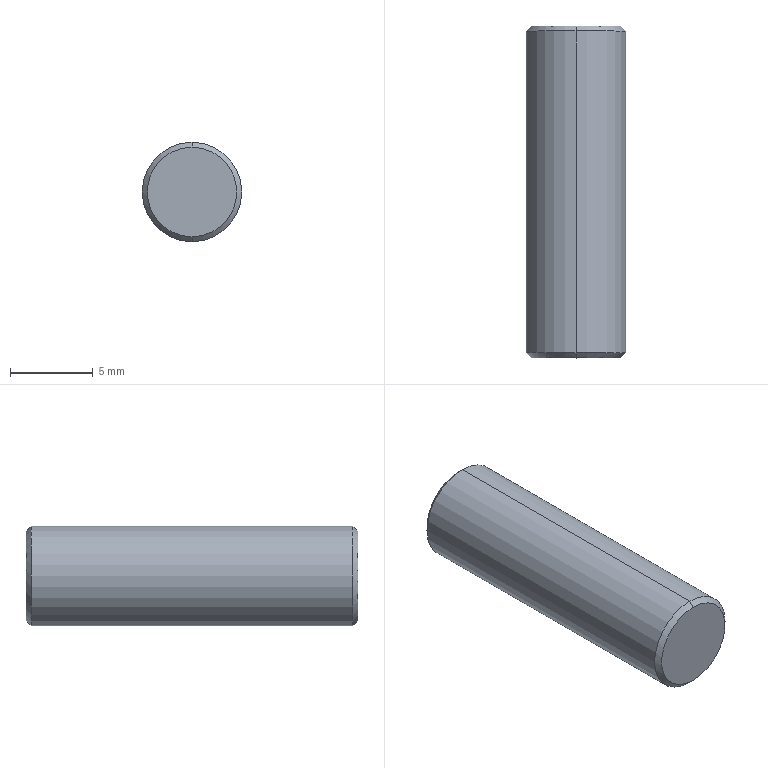Part | STEP file | PN_0030_default | 1 solid | 8 faces | box 6 x 20 x 6 mm | volume 563.847 mm3 | cone 4 | cylinder 2 | plane 2 | commonest cylinder face diameters 6 x2
STEP:
#1=CARTESIAN_POINT('',(0.,0.,0.));
#2=DIRECTION('',(0.,0.,1.));
#3=DIRECTION('',(1.,0.,0.));
#4=AXIS2_PLACEMENT_3D('',#1,#2,#3);
#5=CARTESIAN_POINT('',(0.,20.,2.7));
#6=VERTEX_POINT('',#5);
#7=CARTESIAN_POINT('',(0.,20.,-2.7));
#8=VERTEX_POINT('',#7);
#9=CARTESIAN_POINT('',(0.,20.,0.));
#10=DIRECTION('',(0.,1.,0.));
#11=DIRECTION('',(0.,0.,1.));
#12=AXIS2_PLACEMENT_3D('',#9,#10,#11);
#13=CIRCLE('',#12,2.7);
#14=CARTESIAN_POINT('',(0.,20.,0.));
#15=DIRECTION('',(0.,-1.,0.));
#16=DIRECTION('',(0.,0.,-1.));
#17=AXIS2_PLACEMENT_3D('',#14,#15,#16);
#18=CONICAL_SURFACE('',#17,2.7,0.7854);
#19=CARTESIAN_POINT('',(3.142,0.));
#20=DIRECTION('',(-1.,0.));
#21=VECTOR('',#20,1.);
#22=LINE('',#19,#21);
#23=(GEOMETRIC_REPRESENTATION_CONTEXT(2)PARAMETRIC_REPRESENTATION_CONTEXT()REPRESENTATION_CONTEXT('',''));
#24=DEFINITIONAL_REPRESENTATION('',(#22),#23);
#25=PCURVE('',#18,#24);
#26=CARTESIAN_POINT('',(0.,20.,0.));
#27=DIRECTION('',(0.,1.,0.));
#28=DIRECTION('',(0.,0.,1.));
#29=AXIS2_PLACEMENT_3D('',#26,#27,#28);
#30=PLANE('',#29);
#31=CARTESIAN_POINT('',(0.,0.));
#32=DIRECTION('',(1.,0.));
#33=AXIS2_PLACEMENT_2D('',#31,#32);
#34=CIRCLE('',#33,2.7);
#35=(GEOMETRIC_REPRESENTATION_CONTEXT(2)PARAMETRIC_REPRESENTATION_CONTEXT()REPRESENTATION_CONTEXT('',''));
#36=DEFINITIONAL_REPRESENTATION('',(#34),#35);
#37=PCURVE('',#30,#36);
#38=SURFACE_CURVE('',#13,(#25,#37),.PCURVE_S1.);
#39=EDGE_CURVE('',#6,#8,#38,.T.);
#40=ORIENTED_EDGE('',*,*,#39,.F.);
#41=CARTESIAN_POINT('',(0.,19.7,3.));
#42=VERTEX_POINT('',#41);
#43=CARTESIAN_POINT('',(0.,20.,2.7));
#44=DIRECTION('',(0.,-0.7071,0.7071));
#45=VECTOR('',#44,1.);
#46=LINE('',#43,#45);
#47=CARTESIAN_POINT('',(3.142,0.));
#48=DIRECTION('',(0.,1.));
#49=VECTOR('',#48,1.);
#50=LINE('',#47,#49);
#51=(GEOMETRIC_REPRESENTATION_CONTEXT(2)PARAMETRIC_REPRESENTATION_CONTEXT()REPRESENTATION_CONTEXT('',''));
#52=DEFINITIONAL_REPRESENTATION('',(#50),#51);
#53=PCURVE('',#18,#52);
#54=CARTESIAN_POINT('',(0.,20.,0.));
#55=DIRECTION('',(0.,-1.,0.));
#56=DIRECTION('',(0.,0.,-1.));
#57=AXIS2_PLACEMENT_3D('',#54,#55,#56);
#58=CONICAL_SURFACE('',#57,2.7,0.7854);
#59=CARTESIAN_POINT('',(3.142,0.));
#60=DIRECTION('',(0.,1.));
#61=VECTOR('',#60,1.);
#62=LINE('',#59,#61);
#63=(GEOMETRIC_REPRESENTATION_CONTEXT(2)PARAMETRIC_REPRESENTATION_CONTEXT()REPRESENTATION_CONTEXT('',''));
#64=DEFINITIONAL_REPRESENTATION('',(#62),#63);
#65=PCURVE('',#58,#64);
#66=SURFACE_CURVE('',#46,(#53,#65),.PCURVE_S1.);
#67=EDGE_CURVE('',#6,#42,#66,.T.);
#68=ORIENTED_EDGE('',*,*,#67,.T.);
#69=CARTESIAN_POINT('',(0.,19.7,-3.));
#70=VERTEX_POINT('',#69);
#71=CARTESIAN_POINT('',(0.,19.7,0.));
#72=DIRECTION('',(0.,-1.,0.));
#73=DIRECTION('',(0.,0.,1.));
#74=AXIS2_PLACEMENT_3D('',#71,#72,#73);
#75=CIRCLE('',#74,3.);
#76=CARTESIAN_POINT('',(-3.142,0.3));
#77=DIRECTION('',(1.,0.));
#78=VECTOR('',#77,1.);
#79=LINE('',#76,#78);
#80=(GEOMETRIC_REPRESENTATION_CONTEXT(2)PARAMETRIC_REPRESENTATION_CONTEXT()REPRESENTATION_CONTEXT('',''));
#81=DEFINITIONAL_REPRESENTATION('',(#79),#80);
#82=PCURVE('',#18,#81);
#83=CARTESIAN_POINT('',(0.,20.,0.));
#84=DIRECTION('',(0.,-1.,0.));
#85=DIRECTION('',(0.,0.,-1.));
#86=AXIS2_PLACEMENT_3D('',#83,#84,#85);
#87=CYLINDRICAL_SURFACE('',#86,3.);
#88=CARTESIAN_POINT('',(-3.142,0.3));
#89=DIRECTION('',(1.,0.));
#90=VECTOR('',#89,1.);
#91=LINE('',#88,#90);
#92=(GEOMETRIC_REPRESENTATION_CONTEXT(2)PARAMETRIC_REPRESENTATION_CONTEXT()REPRESENTATION_CONTEXT('',''));
#93=DEFINITIONAL_REPRESENTATION('',(#91),#92);
#94=PCURVE('',#87,#93);
#95=SURFACE_CURVE('',#75,(#82,#94),.PCURVE_S1.);
#96=EDGE_CURVE('',#70,#42,#95,.T.);
#97=ORIENTED_EDGE('',*,*,#96,.F.);
#98=CARTESIAN_POINT('',(0.,20.,-2.7));
#99=DIRECTION('',(0.,-0.7071,-0.7071));
#100=VECTOR('',#99,1.);
#101=LINE('',#98,#100);
#102=CARTESIAN_POINT('',(0.,0.));
#103=DIRECTION('',(0.,1.));
#104=VECTOR('',#103,1.);
#105=LINE('',#102,#104);
#106=(GEOMETRIC_REPRESENTATION_CONTEXT(2)PARAMETRIC_REPRESENTATION_CONTEXT()REPRESENTATION_CONTEXT('',''));
#107=DEFINITIONAL_REPRESENTATION('',(#105),#106);
#108=PCURVE('',#18,#107);
#109=CARTESIAN_POINT('',(6.283,0.));
#110=DIRECTION('',(0.,1.));
#111=VECTOR('',#110,1.);
#112=LINE('',#109,#111);
#113=(GEOMETRIC_REPRESENTATION_CONTEXT(2)PARAMETRIC_REPRESENTATION_CONTEXT()REPRESENTATION_CONTEXT('',''));
#114=DEFINITIONAL_REPRESENTATION('',(#112),#113);
#115=PCURVE('',#58,#114);
#116=SURFACE_CURVE('',#101,(#108,#115),.PCURVE_S1.);
#117=EDGE_CURVE('',#8,#70,#116,.T.);
#118=ORIENTED_EDGE('',*,*,#117,.F.);
#119=EDGE_LOOP('',(#40,#68,#97,#118));
#120=FACE_BOUND('',#119,.T.);
#121=ADVANCED_FACE('',(#120),#18,.T.);
#122=CARTESIAN_POINT('',(0.,0.,-2.7));
#123=VERTEX_POINT('',#122);
#124=CARTESIAN_POINT('',(0.,0.,2.7));
#125=VERTEX_POINT('',#124);
#126=CARTESIAN_POINT('',(0.,0.,0.));
#127=DIRECTION('',(0.,-1.,0.));
#128=DIRECTION('',(0.,0.,1.));
#129=AXIS2_PLACEMENT_3D('',#126,#127,#128);
#130=CIRCLE('',#129,2.7);
#131=CARTESIAN_POINT('',(0.,0.3,0.));
#132=DIRECTION('',(0.,1.,0.));
#133=DIRECTION('',(0.,0.,1.));
#134=AXIS2_PLACEMENT_3D('',#131,#132,#133);
#135=CONICAL_SURFACE('',#134,3.,0.7854);
#136=CARTESIAN_POINT('',(6.283,-0.3));
#137=DIRECTION('',(-1.,0.));
#138=VECTOR('',#137,1.);
#139=LINE('',#136,#138);
#140=(GEOMETRIC_REPRESENTATION_CONTEXT(2)PARAMETRIC_REPRESENTATION_CONTEXT()REPRESENTATION_CONTEXT('',''));
#141=DEFINITIONAL_REPRESENTATION('',(#139),#140);
#142=PCURVE('',#135,#141);
#143=CARTESIAN_POINT('',(0.,0.,0.));
#144=DIRECTION('',(0.,1.,0.));
#145=DIRECTION('',(0.,0.,1.));
#146=AXIS2_PLACEMENT_3D('',#143,#144,#145);
#147=PLANE('',#146);
#148=CARTESIAN_POINT('',(2.7,0.));
#149=CARTESIAN_POINT('',(2.7,-4.677));
#150=CARTESIAN_POINT('',(-1.35,-2.338));
#151=CARTESIAN_POINT('',(-5.4,0.));
#152=CARTESIAN_POINT('',(-1.35,2.338));
#153=CARTESIAN_POINT('',(2.7,4.677));
#154=CARTESIAN_POINT('',(2.7,0.));
#155=(BOUNDED_CURVE()B_SPLINE_CURVE(2,(#148,#149,#150,#151,#152,#153,#154),.UNSPECIFIED.,.T.,.F.)B_SPLINE_CURVE_WITH_KNOTS((1,2,2,2,2,1),(-2.094,0.,2.094,4.189,6.283,8.378),.UNSPECIFIED.)CURVE()GEOMETRIC_REPRESENTATION_ITEM()RATIONAL_B_SPLINE_CURVE((1.,0.5,1.,0.5,1.,0.5,1.))REPRESENTATION_ITEM(''));
#156=(GEOMETRIC_REPRESENTATION_CONTEXT(2)PARAMETRIC_REPRESENTATION_CONTEXT()REPRESENTATION_CONTEXT('',''));
#157=DEFINITIONAL_REPRESENTATION('',(#155),#156);
#158=PCURVE('',#147,#157);
#159=SURFACE_CURVE('',#130,(#142,#158),.PCURVE_S1.);
#160=EDGE_CURVE('',#123,#125,#159,.T.);
#161=ORIENTED_EDGE('',*,*,#160,.F.);
#162=CARTESIAN_POINT('',(0.,0.3,-3.));
#163=VERTEX_POINT('',#162);
#164=CARTESIAN_POINT('',(0.,0.3,-3.));
#165=DIRECTION('',(0.,0.7071,-0.7071));
#166=VECTOR('',#165,1.);
#167=LINE('',#164,#166);
#168=CARTESIAN_POINT('',(3.142,0.));
#169=DIRECTION('',(0.,1.));
#170=VECTOR('',#169,1.);
#171=LINE('',#168,#170);
#172=(GEOMETRIC_REPRESENTATION_CONTEXT(2)PARAMETRIC_REPRESENTATION_CONTEXT()REPRESENTATION_CONTEXT('',''));
#173=DEFINITIONAL_REPRESENTATION('',(#171),#172);
#174=PCURVE('',#135,#173);
#175=CARTESIAN_POINT('',(0.,0.3,0.));
#176=DIRECTION('',(0.,1.,0.));
#177=DIRECTION('',(0.,0.,1.));
#178=AXIS2_PLACEMENT_3D('',#175,#176,#177);
#179=CONICAL_SURFACE('',#178,3.,0.7854);
#180=CARTESIAN_POINT('',(3.142,0.));
#181=DIRECTION('',(0.,1.));
#182=VECTOR('',#181,1.);
#183=LINE('',#180,#182);
#184=(GEOMETRIC_REPRESENTATION_CONTEXT(2)PARAMETRIC_REPRESENTATION_CONTEXT()REPRESENTATION_CONTEXT('',''));
#185=DEFINITIONAL_REPRESENTATION('',(#183),#184);
#186=PCURVE('',#179,#185);
#187=SURFACE_CURVE('',#167,(#174,#186),.PCURVE_S1.);
#188=EDGE_CURVE('',#123,#163,#187,.T.);
#189=ORIENTED_EDGE('',*,*,#188,.T.);
#190=CARTESIAN_POINT('',(0.,0.3,3.));
#191=VERTEX_POINT('',#190);
#192=CARTESIAN_POINT('',(0.,0.3,0.));
#193=DIRECTION('',(0.,1.,0.));
#194=DIRECTION('',(0.,0.,1.));
#195=AXIS2_PLACEMENT_3D('',#192,#193,#194);
#196=CIRCLE('',#195,3.);
#197=CARTESIAN_POINT('',(0.,0.));
#198=DIRECTION('',(1.,0.));
#199=VECTOR('',#198,1.);
#200=LINE('',#197,#199);
#201=(GEOMETRIC_REPRESENTATION_CONTEXT(2)PARAMETRIC_REPRESENTATION_CONTEXT()REPRESENTATION_CONTEXT('',''));
#202=DEFINITIONAL_REPRESENTATION('',(#200),#201);
#203=PCURVE('',#135,#202);
#204=CARTESIAN_POINT('',(3.142,19.7));
#205=DIRECTION('',(-1.,0.));
#206=VECTOR('',#205,1.);
#207=LINE('',#204,#206);
#208=(GEOMETRIC_REPRESENTATION_CONTEXT(2)PARAMETRIC_REPRESENTATION_CONTEXT()REPRESENTATION_CONTEXT('',''));
#209=DEFINITIONAL_REPRESENTATION('',(#207),#208);
#210=PCURVE('',#87,#209);
#211=SURFACE_CURVE('',#196,(#203,#210),.PCURVE_S1.);
#212=EDGE_CURVE('',#191,#163,#211,.T.);
#213=ORIENTED_EDGE('',*,*,#212,.F.);
#214=CARTESIAN_POINT('',(0.,0.3,3.));
#215=DIRECTION('',(0.,0.7071,0.7071));
#216=VECTOR('',#215,1.);
#217=LINE('',#214,#216);
#218=CARTESIAN_POINT('',(0.,0.));
#219=DIRECTION('',(0.,1.));
#220=VECTOR('',#219,1.);
#221=LINE('',#218,#220);
#222=(GEOMETRIC_REPRESENTATION_CONTEXT(2)PARAMETRIC_REPRESENTATION_CONTEXT()REPRESENTATION_CONTEXT('',''));
#223=DEFINITIONAL_REPRESENTATION('',(#221),#222);
#224=PCURVE('',#135,#223);
#225=CARTESIAN_POINT('',(6.283,0.));
#226=DIRECTION('',(0.,1.));
#227=VECTOR('',#226,1.);
#228=LINE('',#225,#227);
#229=(GEOMETRIC_REPRESENTATION_CONTEXT(2)PARAMETRIC_REPRESENTATION_CONTEXT()REPRESENTATION_CONTEXT('',''));
#230=DEFINITIONAL_REPRESENTATION('',(#228),#229);
#231=PCURVE('',#179,#230);
#232=SURFACE_CURVE('',#217,(#224,#231),.PCURVE_S1.);
#233=EDGE_CURVE('',#125,#191,#232,.T.);
#234=ORIENTED_EDGE('',*,*,#233,.F.);
#235=EDGE_LOOP('',(#161,#189,#213,#234));
#236=FACE_BOUND('',#235,.T.);
#237=ADVANCED_FACE('',(#236),#135,.T.);
#238=ORIENTED_EDGE('',*,*,#96,.T.);
#239=CARTESIAN_POINT('',(0.,20.,3.));
#240=DIRECTION('',(0.,-1.,0.));
#241=VECTOR('',#240,1.);
#242=LINE('',#239,#241);
#243=CARTESIAN_POINT('',(3.142,0.));
#244=DIRECTION('',(0.,1.));
#245=VECTOR('',#244,1.);
#246=LINE('',#243,#245);
#247=(GEOMETRIC_REPRESENTATION_CONTEXT(2)PARAMETRIC_REPRESENTATION_CONTEXT()REPRESENTATION_CONTEXT('',''));
#248=DEFINITIONAL_REPRESENTATION('',(#246),#247);
#249=PCURVE('',#87,#248);
#250=CARTESIAN_POINT('',(0.,20.,0.));
#251=DIRECTION('',(0.,-1.,0.));
#252=DIRECTION('',(0.,0.,-1.));
#253=AXIS2_PLACEMENT_3D('',#250,#251,#252);
#254=CYLINDRICAL_SURFACE('',#253,3.);
#255=CARTESIAN_POINT('',(3.142,0.));
#256=DIRECTION('',(0.,1.));
#257=VECTOR('',#256,1.);
#258=LINE('',#255,#257);
#259=(GEOMETRIC_REPRESENTATION_CONTEXT(2)PARAMETRIC_REPRESENTATION_CONTEXT()REPRESENTATION_CONTEXT('',''));
#260=DEFINITIONAL_REPRESENTATION('',(#258),#259);
#261=PCURVE('',#254,#260);
#262=SURFACE_CURVE('',#242,(#249,#261),.PCURVE_S1.);
#263=EDGE_CURVE('',#42,#191,#262,.T.);
#264=ORIENTED_EDGE('',*,*,#263,.T.);
#265=ORIENTED_EDGE('',*,*,#212,.T.);
#266=CARTESIAN_POINT('',(0.,20.,-3.));
#267=DIRECTION('',(0.,-1.,0.));
#268=VECTOR('',#267,1.);
#269=LINE('',#266,#268);
#270=CARTESIAN_POINT('',(0.,0.));
#271=DIRECTION('',(0.,1.));
#272=VECTOR('',#271,1.);
#273=LINE('',#270,#272);
#274=(GEOMETRIC_REPRESENTATION_CONTEXT(2)PARAMETRIC_REPRESENTATION_CONTEXT()REPRESENTATION_CONTEXT('',''));
#275=DEFINITIONAL_REPRESENTATION('',(#273),#274);
#276=PCURVE('',#87,#275);
#277=CARTESIAN_POINT('',(6.283,0.));
#278=DIRECTION('',(0.,1.));
#279=VECTOR('',#278,1.);
#280=LINE('',#277,#279);
#281=(GEOMETRIC_REPRESENTATION_CONTEXT(2)PARAMETRIC_REPRESENTATION_CONTEXT()REPRESENTATION_CONTEXT('',''));
#282=DEFINITIONAL_REPRESENTATION('',(#280),#281);
#283=PCURVE('',#254,#282);
#284=SURFACE_CURVE('',#269,(#276,#283),.PCURVE_S1.);
#285=EDGE_CURVE('',#70,#163,#284,.T.);
#286=ORIENTED_EDGE('',*,*,#285,.F.);
#287=EDGE_LOOP('',(#238,#264,#265,#286));
#288=FACE_BOUND('',#287,.T.);
#289=ADVANCED_FACE('',(#288),#87,.T.);
#290=ORIENTED_EDGE('',*,*,#263,.F.);
#291=CARTESIAN_POINT('',(0.,19.7,0.));
#292=DIRECTION('',(0.,-1.,0.));
#293=DIRECTION('',(0.,0.,1.));
#294=AXIS2_PLACEMENT_3D('',#291,#292,#293);
#295=CIRCLE('',#294,3.);
#296=CARTESIAN_POINT('',(3.142,0.3));
#297=DIRECTION('',(1.,0.));
#298=VECTOR('',#297,1.);
#299=LINE('',#296,#298);
#300=(GEOMETRIC_REPRESENTATION_CONTEXT(2)PARAMETRIC_REPRESENTATION_CONTEXT()REPRESENTATION_CONTEXT('',''));
#301=DEFINITIONAL_REPRESENTATION('',(#299),#300);
#302=PCURVE('',#254,#301);
#303=CARTESIAN_POINT('',(3.142,0.3));
#304=DIRECTION('',(1.,0.));
#305=VECTOR('',#304,1.);
#306=LINE('',#303,#305);
#307=(GEOMETRIC_REPRESENTATION_CONTEXT(2)PARAMETRIC_REPRESENTATION_CONTEXT()REPRESENTATION_CONTEXT('',''));
#308=DEFINITIONAL_REPRESENTATION('',(#306),#307);
#309=PCURVE('',#58,#308);
#310=SURFACE_CURVE('',#295,(#302,#309),.PCURVE_S1.);
#311=EDGE_CURVE('',#42,#70,#310,.T.);
#312=ORIENTED_EDGE('',*,*,#311,.T.);
#313=ORIENTED_EDGE('',*,*,#285,.T.);
#314=CARTESIAN_POINT('',(0.,0.3,0.));
#315=DIRECTION('',(0.,1.,0.));
#316=DIRECTION('',(0.,0.,1.));
#317=AXIS2_PLACEMENT_3D('',#314,#315,#316);
#318=CIRCLE('',#317,3.);
#319=CARTESIAN_POINT('',(9.425,19.7));
#320=DIRECTION('',(-1.,0.));
#321=VECTOR('',#320,1.);
#322=LINE('',#319,#321);
#323=(GEOMETRIC_REPRESENTATION_CONTEXT(2)PARAMETRIC_REPRESENTATION_CONTEXT()REPRESENTATION_CONTEXT('',''));
#324=DEFINITIONAL_REPRESENTATION('',(#322),#323);
#325=PCURVE('',#254,#324);
#326=CARTESIAN_POINT('',(0.,0.));
#327=DIRECTION('',(1.,0.));
#328=VECTOR('',#327,1.);
#329=LINE('',#326,#328);
#330=(GEOMETRIC_REPRESENTATION_CONTEXT(2)PARAMETRIC_REPRESENTATION_CONTEXT()REPRESENTATION_CONTEXT('',''));
#331=DEFINITIONAL_REPRESENTATION('',(#329),#330);
#332=PCURVE('',#179,#331);
#333=SURFACE_CURVE('',#318,(#325,#332),.PCURVE_S1.);
#334=EDGE_CURVE('',#163,#191,#333,.T.);
#335=ORIENTED_EDGE('',*,*,#334,.T.);
#336=EDGE_LOOP('',(#290,#312,#313,#335));
#337=FACE_BOUND('',#336,.T.);
#338=ADVANCED_FACE('',(#337),#254,.T.);
#339=CARTESIAN_POINT('',(0.,20.,0.));
#340=DIRECTION('',(0.,1.,0.));
#341=DIRECTION('',(0.,0.,1.));
#342=AXIS2_PLACEMENT_3D('',#339,#340,#341);
#343=CIRCLE('',#342,2.7);
#344=CARTESIAN_POINT('',(0.,0.));
#345=DIRECTION('',(1.,0.));
#346=AXIS2_PLACEMENT_2D('',#344,#345);
#347=CIRCLE('',#346,2.7);
#348=(GEOMETRIC_REPRESENTATION_CONTEXT(2)PARAMETRIC_REPRESENTATION_CONTEXT()REPRESENTATION_CONTEXT('',''));
#349=DEFINITIONAL_REPRESENTATION('',(#347),#348);
#350=PCURVE('',#30,#349);
#351=CARTESIAN_POINT('',(9.425,0.));
#352=DIRECTION('',(-1.,0.));
#353=VECTOR('',#352,1.);
#354=LINE('',#351,#353);
#355=(GEOMETRIC_REPRESENTATION_CONTEXT(2)PARAMETRIC_REPRESENTATION_CONTEXT()REPRESENTATION_CONTEXT('',''));
#356=DEFINITIONAL_REPRESENTATION('',(#354),#355);
#357=PCURVE('',#58,#356);
#358=SURFACE_CURVE('',#343,(#350,#357),.PCURVE_S1.);
#359=EDGE_CURVE('',#8,#6,#358,.T.);
#360=ORIENTED_EDGE('',*,*,#359,.T.);
#361=ORIENTED_EDGE('',*,*,#39,.T.);
#362=EDGE_LOOP('',(#360,#361));
#363=FACE_BOUND('',#362,.T.);
#364=ADVANCED_FACE('',(#363),#30,.T.);
#365=CARTESIAN_POINT('',(0.,0.,0.));
#366=DIRECTION('',(0.,-1.,0.));
#367=DIRECTION('',(0.,0.,1.));
#368=AXIS2_PLACEMENT_3D('',#365,#366,#367);
#369=CIRCLE('',#368,2.7);
#370=CARTESIAN_POINT('',(2.7,0.));
#371=CARTESIAN_POINT('',(2.7,-4.677));
#372=CARTESIAN_POINT('',(-1.35,-2.338));
#373=CARTESIAN_POINT('',(-5.4,0.));
#374=CARTESIAN_POINT('',(-1.35,2.338));
#375=CARTESIAN_POINT('',(2.7,4.677));
#376=CARTESIAN_POINT('',(2.7,0.));
#377=(BOUNDED_CURVE()B_SPLINE_CURVE(2,(#370,#371,#372,#373,#374,#375,#376),.UNSPECIFIED.,.T.,.F.)B_SPLINE_CURVE_WITH_KNOTS((1,2,2,2,2,1),(-2.094,0.,2.094,4.189,6.283,8.378),.UNSPECIFIED.)CURVE()GEOMETRIC_REPRESENTATION_ITEM()RATIONAL_B_SPLINE_CURVE((1.,0.5,1.,0.5,1.,0.5,1.))REPRESENTATION_ITEM(''));
#378=(GEOMETRIC_REPRESENTATION_CONTEXT(2)PARAMETRIC_REPRESENTATION_CONTEXT()REPRESENTATION_CONTEXT('',''));
#379=DEFINITIONAL_REPRESENTATION('',(#377),#378);
#380=PCURVE('',#147,#379);
#381=CARTESIAN_POINT('',(6.283,-0.3));
#382=DIRECTION('',(-1.,0.));
#383=VECTOR('',#382,1.);
#384=LINE('',#381,#383);
#385=(GEOMETRIC_REPRESENTATION_CONTEXT(2)PARAMETRIC_REPRESENTATION_CONTEXT()REPRESENTATION_CONTEXT('',''));
#386=DEFINITIONAL_REPRESENTATION('',(#384),#385);
#387=PCURVE('',#179,#386);
#388=SURFACE_CURVE('',#369,(#380,#387),.PCURVE_S1.);
#389=EDGE_CURVE('',#125,#123,#388,.T.);
#390=ORIENTED_EDGE('',*,*,#389,.T.);
#391=ORIENTED_EDGE('',*,*,#160,.T.);
#392=EDGE_LOOP('',(#390,#391));
#393=FACE_BOUND('',#392,.T.);
#394=ADVANCED_FACE('',(#393),#147,.F.);
#395=ORIENTED_EDGE('',*,*,#188,.F.);
#396=ORIENTED_EDGE('',*,*,#389,.F.);
#397=ORIENTED_EDGE('',*,*,#233,.T.);
#398=ORIENTED_EDGE('',*,*,#334,.F.);
#399=EDGE_LOOP('',(#395,#396,#397,#398));
#400=FACE_BOUND('',#399,.T.);
#401=ADVANCED_FACE('',(#400),#179,.T.);
#402=ORIENTED_EDGE('',*,*,#67,.F.);
#403=ORIENTED_EDGE('',*,*,#359,.F.);
#404=ORIENTED_EDGE('',*,*,#117,.T.);
#405=ORIENTED_EDGE('',*,*,#311,.F.);
#406=EDGE_LOOP('',(#402,#403,#404,#405));
#407=FACE_BOUND('',#406,.T.);
#408=ADVANCED_FACE('',(#407),#58,.T.);
#409=CLOSED_SHELL('',(#121,#237,#289,#338,#364,#394,#401,#408));
#410=MANIFOLD_SOLID_BREP('',#409);
#411=(LENGTH_UNIT()NAMED_UNIT(*)SI_UNIT(.MILLI.,.METRE.));
#412=UNCERTAINTY_MEASURE_WITH_UNIT(LENGTH_MEASURE(0.0000001),#411,'','');
#413=(NAMED_UNIT(*)PLANE_ANGLE_UNIT()SI_UNIT($,.RADIAN.));
#414=(NAMED_UNIT(*)SI_UNIT($,.STERADIAN.)SOLID_ANGLE_UNIT());
#415=(GEOMETRIC_REPRESENTATION_CONTEXT(3)GLOBAL_UNCERTAINTY_ASSIGNED_CONTEXT((#412))GLOBAL_UNIT_ASSIGNED_CONTEXT((#411,#413,#414))REPRESENTATION_CONTEXT('',''));
#416=ADVANCED_BREP_SHAPE_REPRESENTATION('',(#4,#410),#415);